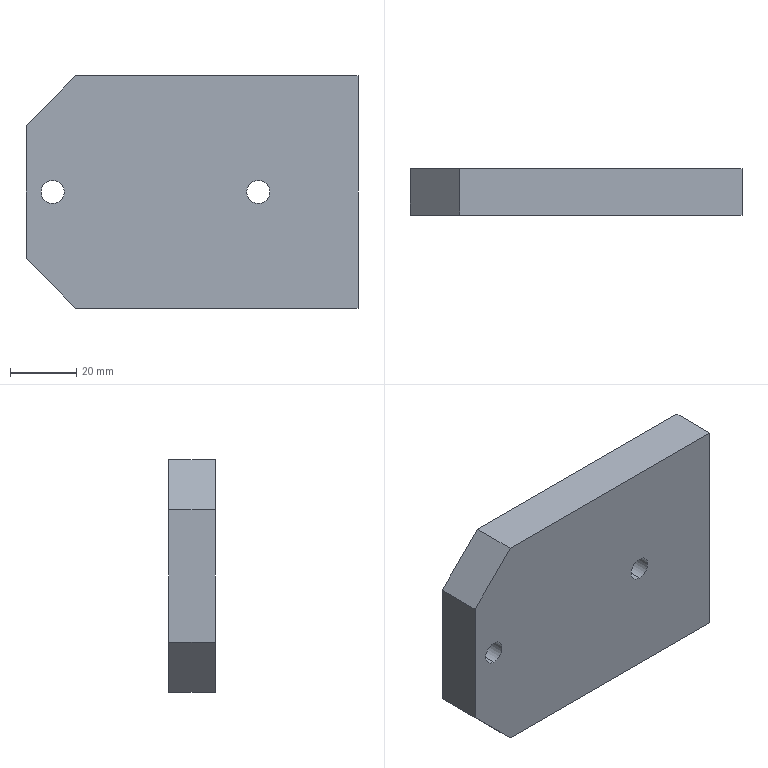Part | STEP file | OP10-132_side plate (2)-L | 1 solid | 30 faces | box 100 x 14 x 70 mm | volume 92004 mm3 | cylinder 14 | plane 10 | cone 6 | commonest cylinder face diameters 5 x6 7 x4 11 x4